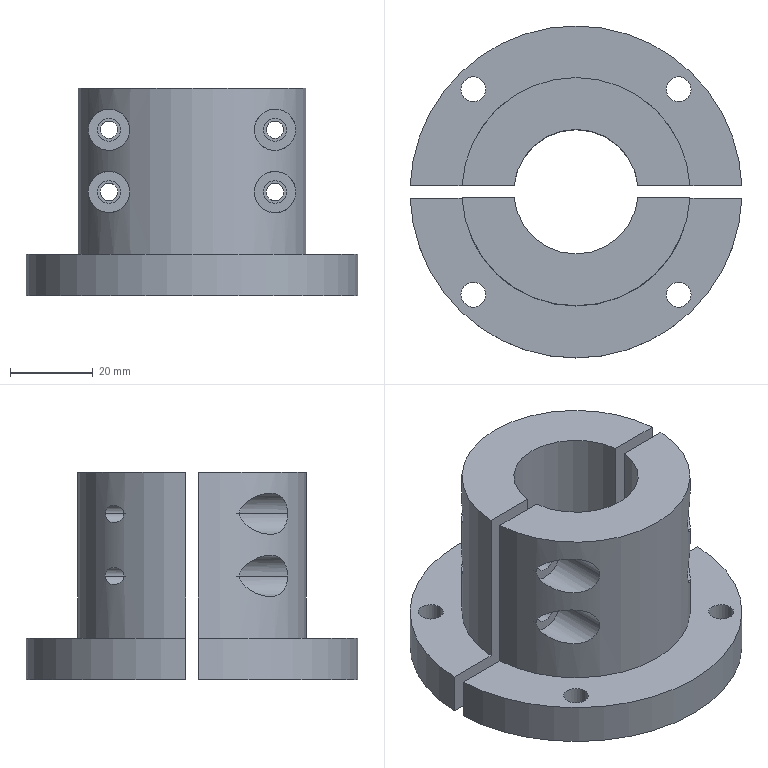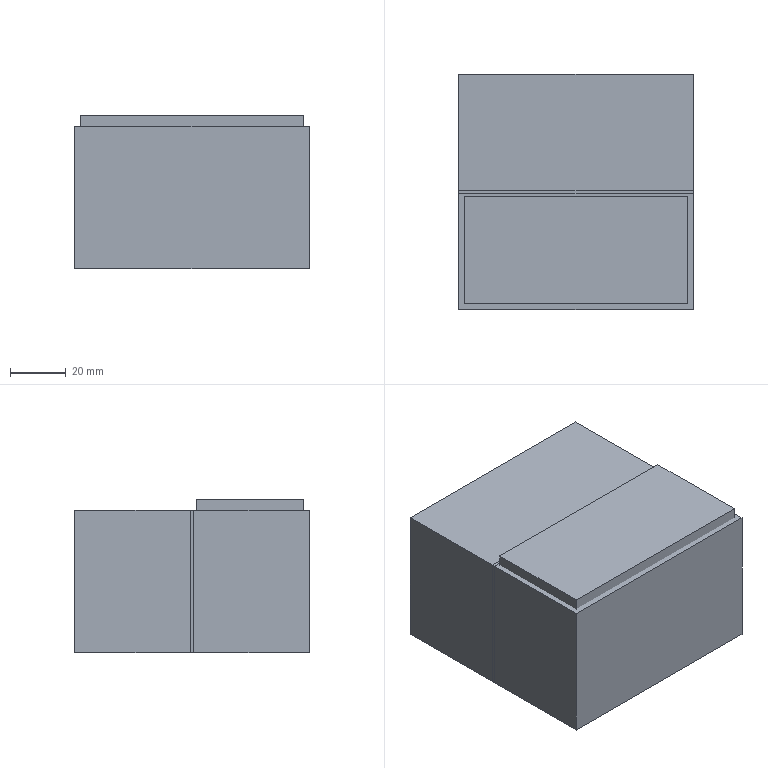CAM job | NX | 3+2 milling, drilling | part box 79.944 x 80 x 50 mm | stock box 83.944 x 84 x 55 mm
Tools:
number,name,description,diameter,corner_radius,flute_length,length,flutes
19,D80,Milling Tool-5 Parameters,80.0,0.0,50.0,75.0,2
15,D10,Milling Tool-5 Parameters,10.0,0.0,50.0,75.0,2
14,D10JING,Milling Tool-5 Parameters,10.0,0.0,50.0,75.0,2
1,D6A45,Milling Tool-5 Parameters,6.0,0.0,50.0,75.0,2
4,4.2ZT,Drilling Tool,4.2,0.0,35.0,50.0,2
16,6.0ZT,Drilling Tool,6.0,0.0,35.0,50.0,2
12,D6,Milling Tool-5 Parameters,6.0,0.0,50.0,75.0,2
9,5.5ZT,Drilling Tool,5.5,0.0,35.0,50.0,2
17,D3,Milling Tool-5 Parameters,3.0,0.0,50.0,75.0,2
18,D4A45,Milling Tool-5 Parameters,4.0,0.0,50.0,75.0,2
Operations:
program,operation,operation_type,tool,method,geometry_group,spindle_rpm,surface_speed,feed_per_tooth,feed_cut,feed_plunge,cut_length_mm,path_length_mm,cut_time_min,machine_time_min
1共用,FLOOR_WALL_COPY,VolumeBased25DMillingOperation,D80,METHOD,A,6500.0,1633.0,0.1154,1500.0,100.0,179.944,233.944,0.12,0.1254
1共用,CAVITY_MILL,CavityMilling,D10,METHOD,A,9500.0,298.0,0.1316,2500.0,1000.0,39274.748,40185.253,16,16.091
1共用,ZLEVEL_PROFILE_COPY_1_COPY_COPY_1,ZLevelMilling,D10JING,METHOD,A,9500.0,298.0,0.0632,1200.0,1000.0,581.217,1430.32,0.4881,0.573
1共用,ZLEVEL_PROFILE_COPY_1_COPY_COPY_1_COPY,ZLevelMilling,D10JING,METHOD,A,9500.0,298.0,0.0632,1200.0,1000.0,211.292,369.292,0.1767,0.1925
1共用,FLOOR_WALL_1,VolumeBased25DMillingOperation,D10JING,METHOD,A,9500.0,119.0,0.0658,1250.0,100.0,657.979,934.815,0.5264,0.5541
1共用,PLANAR_MILL_COPY_COPY_COPY_COPY_COPY_COPY_1,PlanarMilling,D6A45,METHOD,A,9500.0,179.0,0.0658,1250.0,100.0,164.78,223.78,0.1318,0.1377
1共用,PLANAR_MILL_COPY_COPY_COPY_COPY_COPY_COPY_1_COPY,PlanarMilling,D6A45,METHOD,A,9500.0,179.0,0.0658,1250.0,100.0,152.847,291.847,0.1223,0.1362
1共用,刀补,ZLevelMilling,D10JING,METHOD,A,9500.0,298.0,0.0632,1200.0,1000.0,182.934,838.3,0.1555,0.221
2共用,FLOOR_WALL_COPY_COPY,VolumeBased25DMillingOperation,D80,METHOD,B,6500.0,1633.0,0.1154,1500.0,100.0,879.719,1809.495,0.5865,0.6795
2共用,DRILLING_COPY_1,Operation,D6A45,METHOD,B,5000.0,94.0,0.035,350.0,0.0,8.0,128.588,0.0229,0.0349
2共用,DRILLING_COPY_1_COPY_COPY,Operation,6.0ZT,METHOD,B,2000.0,28.0,0.05,200.0,0.0,32.605,177.799,0.163,0.1775
2共用,PLANAR_MILL_COPY_COPY_COPY_COPY_COPY_COPY_1_COPY_COPY,PlanarMilling,D6A45,METHOD,B,9500.0,179.0,0.0658,1250.0,100.0,264.203,525.553,0.2114,0.2375
3,HOLE_MILLING,CylinderMilling,D6,METHOD,C,9500.0,179.0,0.0789,1500.0,100.0,1539.167,2034.971,1.026,1.076
3,DRILLING_COPY_1_COPY,Operation,D6A45,METHOD,C,5000.0,94.0,0.035,350.0,0.0,16.0,232.707,0.0457,0.0674
3,DRILLING_COPY_1_COPY_COPY_COPY,Operation,5.5ZT,METHOD,C,2000.0,28.0,0.05,200.0,0.0,56.609,313.925,0.283,0.3088
4,HOLE_MILLING_1,CylinderMilling,D3,METHOD,D,9500.0,89.0,0.0658,1250.0,100.0,475.645,954.631,0.3805,0.4284
4,DRILLING_COPY_1_COPY_1,Operation,D4A45,METHOD,D,5000.0,94.0,0.035,350.0,0.0,16.0,219.953,0.0457,0.0661
4,DRILLING_COPY_1_COPY_COPY_1,Operation,4.2ZT,METHOD,D,2000.0,28.0,0.05,200.0,0.0,100.554,379.062,0.5028,0.5306